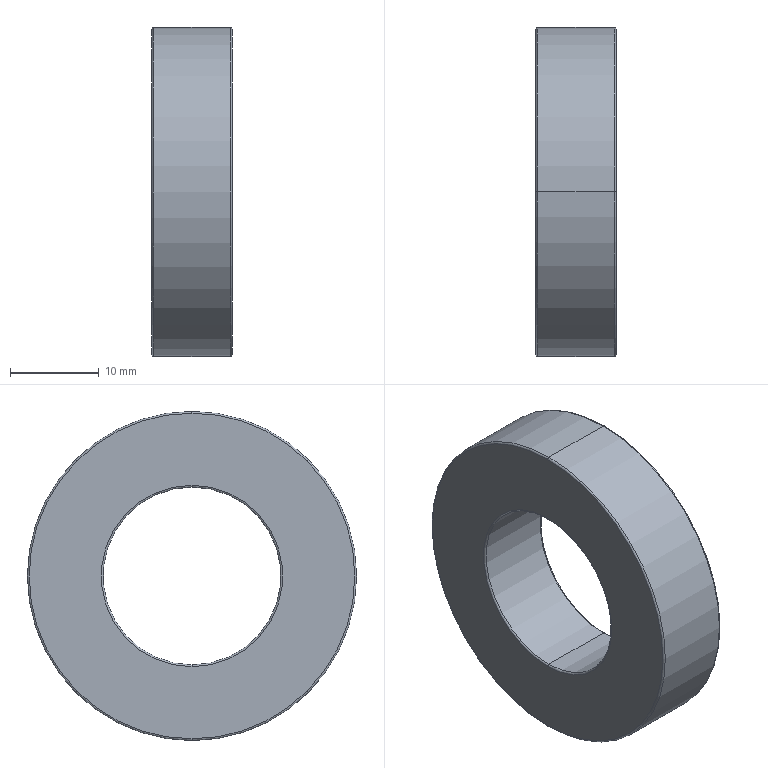Part | SolidWorks | features BaseBody 1 | 1 solid | 14 faces | box 9 x 37 x 37 mm | volume 6846 mm3 | torus 8 | cylinder 4 | plane 2 | commonest cylinder face diameters 20 x2 37 x2
STEP:
#1=CARTESIAN_POINT('',(4.3,0.,18.5));
#2=VERTEX_POINT('',#1);
#3=CARTESIAN_POINT('',(4.3,0.,-18.5));
#4=VERTEX_POINT('',#3);
#5=CARTESIAN_POINT('',(4.3,0.,0.));
#6=DIRECTION('',(-1.,0.,0.));
#7=DIRECTION('',(0.,0.,-1.));
#8=AXIS2_PLACEMENT_3D('',#5,#6,#7);
#9=CIRCLE('',#8,18.5);
#10=EDGE_CURVE('',#2,#4,#9,.T.);
#11=ORIENTED_EDGE('',*,*,#10,.F.);
#12=CARTESIAN_POINT('',(4.5,0.,18.3));
#13=VERTEX_POINT('',#12);
#14=CARTESIAN_POINT('',(4.3,0.,18.3));
#15=DIRECTION('',(0.,1.,0.));
#16=DIRECTION('',(0.,0.,1.));
#17=AXIS2_PLACEMENT_3D('',#14,#15,#16);
#18=CIRCLE('',#17,0.2);
#19=EDGE_CURVE('',#2,#13,#18,.T.);
#20=ORIENTED_EDGE('',*,*,#19,.T.);
#21=CARTESIAN_POINT('',(4.5,0.,-18.3));
#22=VERTEX_POINT('',#21);
#23=CARTESIAN_POINT('',(4.5,0.,0.));
#24=DIRECTION('',(1.,0.,0.));
#25=DIRECTION('',(0.,0.,-1.));
#26=AXIS2_PLACEMENT_3D('',#23,#24,#25);
#27=CIRCLE('',#26,18.3);
#28=EDGE_CURVE('',#22,#13,#27,.T.);
#29=ORIENTED_EDGE('',*,*,#28,.F.);
#30=CARTESIAN_POINT('',(4.3,0.,-18.3));
#31=DIRECTION('',(0.,-1.,0.));
#32=DIRECTION('',(0.,0.,-1.));
#33=AXIS2_PLACEMENT_3D('',#30,#31,#32);
#34=CIRCLE('',#33,0.2);
#35=EDGE_CURVE('',#4,#22,#34,.T.);
#36=ORIENTED_EDGE('',*,*,#35,.F.);
#37=EDGE_LOOP('',(#11,#20,#29,#36));
#38=FACE_OUTER_BOUND('',#37,.T.);
#39=CARTESIAN_POINT('',(4.3,0.,0.));
#40=DIRECTION('',(1.,0.,0.));
#41=DIRECTION('',(0.,0.,-1.));
#42=AXIS2_PLACEMENT_3D('',#39,#40,#41);
#43=TOROIDAL_SURFACE('',#42,18.3,0.2);
#44=ADVANCED_FACE('',(#38),#43,.T.);
#45=CARTESIAN_POINT('',(4.5,0.,10.2));
#46=VERTEX_POINT('',#45);
#47=CARTESIAN_POINT('',(4.5,0.,-10.2));
#48=VERTEX_POINT('',#47);
#49=CARTESIAN_POINT('',(4.5,0.,0.));
#50=DIRECTION('',(-1.,0.,0.));
#51=DIRECTION('',(0.,0.,-1.));
#52=AXIS2_PLACEMENT_3D('',#49,#50,#51);
#53=CIRCLE('',#52,10.2);
#54=EDGE_CURVE('',#46,#48,#53,.T.);
#55=ORIENTED_EDGE('',*,*,#54,.F.);
#56=CARTESIAN_POINT('',(4.3,0.,10.));
#57=VERTEX_POINT('',#56);
#58=CARTESIAN_POINT('',(4.3,0.,10.2));
#59=DIRECTION('',(0.,1.,0.));
#60=DIRECTION('',(0.,0.,1.));
#61=AXIS2_PLACEMENT_3D('',#58,#59,#60);
#62=CIRCLE('',#61,0.2);
#63=EDGE_CURVE('',#46,#57,#62,.T.);
#64=ORIENTED_EDGE('',*,*,#63,.T.);
#65=CARTESIAN_POINT('',(4.3,0.,-10.));
#66=VERTEX_POINT('',#65);
#67=CARTESIAN_POINT('',(4.3,0.,0.));
#68=DIRECTION('',(1.,0.,0.));
#69=DIRECTION('',(0.,0.,-1.));
#70=AXIS2_PLACEMENT_3D('',#67,#68,#69);
#71=CIRCLE('',#70,10.);
#72=EDGE_CURVE('',#66,#57,#71,.T.);
#73=ORIENTED_EDGE('',*,*,#72,.F.);
#74=CARTESIAN_POINT('',(4.3,0.,-10.2));
#75=DIRECTION('',(0.,-1.,0.));
#76=DIRECTION('',(0.,0.,-1.));
#77=AXIS2_PLACEMENT_3D('',#74,#75,#76);
#78=CIRCLE('',#77,0.2);
#79=EDGE_CURVE('',#48,#66,#78,.T.);
#80=ORIENTED_EDGE('',*,*,#79,.F.);
#81=EDGE_LOOP('',(#55,#64,#73,#80));
#82=FACE_OUTER_BOUND('',#81,.T.);
#83=CARTESIAN_POINT('',(4.3,0.,0.));
#84=DIRECTION('',(1.,0.,0.));
#85=DIRECTION('',(0.,0.,-1.));
#86=AXIS2_PLACEMENT_3D('',#83,#84,#85);
#87=TOROIDAL_SURFACE('',#86,10.2,0.2);
#88=ADVANCED_FACE('',(#82),#87,.T.);
#89=CARTESIAN_POINT('',(-4.5,0.,18.3));
#90=VERTEX_POINT('',#89);
#91=CARTESIAN_POINT('',(-4.5,0.,-18.3));
#92=VERTEX_POINT('',#91);
#93=CARTESIAN_POINT('',(-4.5,0.,0.));
#94=DIRECTION('',(-1.,0.,0.));
#95=DIRECTION('',(0.,0.,-1.));
#96=AXIS2_PLACEMENT_3D('',#93,#94,#95);
#97=CIRCLE('',#96,18.3);
#98=EDGE_CURVE('',#90,#92,#97,.T.);
#99=ORIENTED_EDGE('',*,*,#98,.F.);
#100=CARTESIAN_POINT('',(-4.3,0.,18.5));
#101=VERTEX_POINT('',#100);
#102=CARTESIAN_POINT('',(-4.3,0.,18.3));
#103=DIRECTION('',(0.,1.,0.));
#104=DIRECTION('',(0.,0.,1.));
#105=AXIS2_PLACEMENT_3D('',#102,#103,#104);
#106=CIRCLE('',#105,0.2);
#107=EDGE_CURVE('',#90,#101,#106,.T.);
#108=ORIENTED_EDGE('',*,*,#107,.T.);
#109=CARTESIAN_POINT('',(-4.3,0.,-18.5));
#110=VERTEX_POINT('',#109);
#111=CARTESIAN_POINT('',(-4.3,0.,0.));
#112=DIRECTION('',(1.,0.,0.));
#113=DIRECTION('',(0.,0.,-1.));
#114=AXIS2_PLACEMENT_3D('',#111,#112,#113);
#115=CIRCLE('',#114,18.5);
#116=EDGE_CURVE('',#110,#101,#115,.T.);
#117=ORIENTED_EDGE('',*,*,#116,.F.);
#118=CARTESIAN_POINT('',(-4.3,0.,-18.3));
#119=DIRECTION('',(0.,-1.,0.));
#120=DIRECTION('',(0.,0.,-1.));
#121=AXIS2_PLACEMENT_3D('',#118,#119,#120);
#122=CIRCLE('',#121,0.2);
#123=EDGE_CURVE('',#92,#110,#122,.T.);
#124=ORIENTED_EDGE('',*,*,#123,.F.);
#125=EDGE_LOOP('',(#99,#108,#117,#124));
#126=FACE_OUTER_BOUND('',#125,.T.);
#127=CARTESIAN_POINT('',(-4.3,0.,0.));
#128=DIRECTION('',(1.,0.,0.));
#129=DIRECTION('',(0.,0.,-1.));
#130=AXIS2_PLACEMENT_3D('',#127,#128,#129);
#131=TOROIDAL_SURFACE('',#130,18.3,0.2);
#132=ADVANCED_FACE('',(#126),#131,.T.);
#133=CARTESIAN_POINT('',(-4.3,0.,10.));
#134=VERTEX_POINT('',#133);
#135=CARTESIAN_POINT('',(-4.3,0.,-10.));
#136=VERTEX_POINT('',#135);
#137=CARTESIAN_POINT('',(-4.3,0.,0.));
#138=DIRECTION('',(-1.,0.,0.));
#139=DIRECTION('',(0.,0.,-1.));
#140=AXIS2_PLACEMENT_3D('',#137,#138,#139);
#141=CIRCLE('',#140,10.);
#142=EDGE_CURVE('',#134,#136,#141,.T.);
#143=ORIENTED_EDGE('',*,*,#142,.F.);
#144=CARTESIAN_POINT('',(-4.5,0.,10.2));
#145=VERTEX_POINT('',#144);
#146=CARTESIAN_POINT('',(-4.3,0.,10.2));
#147=DIRECTION('',(0.,1.,0.));
#148=DIRECTION('',(0.,0.,1.));
#149=AXIS2_PLACEMENT_3D('',#146,#147,#148);
#150=CIRCLE('',#149,0.2);
#151=EDGE_CURVE('',#134,#145,#150,.T.);
#152=ORIENTED_EDGE('',*,*,#151,.T.);
#153=CARTESIAN_POINT('',(-4.5,0.,-10.2));
#154=VERTEX_POINT('',#153);
#155=CARTESIAN_POINT('',(-4.5,0.,0.));
#156=DIRECTION('',(1.,0.,0.));
#157=DIRECTION('',(0.,0.,-1.));
#158=AXIS2_PLACEMENT_3D('',#155,#156,#157);
#159=CIRCLE('',#158,10.2);
#160=EDGE_CURVE('',#154,#145,#159,.T.);
#161=ORIENTED_EDGE('',*,*,#160,.F.);
#162=CARTESIAN_POINT('',(-4.3,0.,-10.2));
#163=DIRECTION('',(0.,-1.,0.));
#164=DIRECTION('',(0.,0.,-1.));
#165=AXIS2_PLACEMENT_3D('',#162,#163,#164);
#166=CIRCLE('',#165,0.2);
#167=EDGE_CURVE('',#136,#154,#166,.T.);
#168=ORIENTED_EDGE('',*,*,#167,.F.);
#169=EDGE_LOOP('',(#143,#152,#161,#168));
#170=FACE_OUTER_BOUND('',#169,.T.);
#171=CARTESIAN_POINT('',(-4.3,0.,0.));
#172=DIRECTION('',(1.,0.,0.));
#173=DIRECTION('',(0.,0.,-1.));
#174=AXIS2_PLACEMENT_3D('',#171,#172,#173);
#175=TOROIDAL_SURFACE('',#174,10.2,0.2);
#176=ADVANCED_FACE('',(#170),#175,.T.);
#177=CARTESIAN_POINT('',(4.3,0.,0.));
#178=DIRECTION('',(1.,0.,0.));
#179=DIRECTION('',(0.,0.,-1.));
#180=AXIS2_PLACEMENT_3D('',#177,#178,#179);
#181=CIRCLE('',#180,10.);
#182=EDGE_CURVE('',#57,#66,#181,.T.);
#183=ORIENTED_EDGE('',*,*,#182,.T.);
#184=CARTESIAN_POINT('',(4.5,0.,-10.));
#185=DIRECTION('',(-1.,0.,0.));
#186=VECTOR('',#185,1000.);
#187=LINE('',#184,#186);
#188=EDGE_CURVE('',#66,#136,#187,.T.);
#189=ORIENTED_EDGE('',*,*,#188,.T.);
#190=CARTESIAN_POINT('',(-4.3,0.,0.));
#191=DIRECTION('',(-1.,0.,0.));
#192=DIRECTION('',(0.,0.,-1.));
#193=AXIS2_PLACEMENT_3D('',#190,#191,#192);
#194=CIRCLE('',#193,10.);
#195=EDGE_CURVE('',#136,#134,#194,.T.);
#196=ORIENTED_EDGE('',*,*,#195,.T.);
#197=CARTESIAN_POINT('',(4.5,0.,10.));
#198=DIRECTION('',(-1.,0.,0.));
#199=VECTOR('',#198,1000.);
#200=LINE('',#197,#199);
#201=EDGE_CURVE('',#57,#134,#200,.T.);
#202=ORIENTED_EDGE('',*,*,#201,.F.);
#203=EDGE_LOOP('',(#183,#189,#196,#202));
#204=FACE_OUTER_BOUND('',#203,.T.);
#205=CARTESIAN_POINT('',(4.5,0.,0.));
#206=DIRECTION('',(-1.,0.,0.));
#207=DIRECTION('',(0.,0.,1.));
#208=AXIS2_PLACEMENT_3D('',#205,#206,#207);
#209=CYLINDRICAL_SURFACE('',#208,10.);
#210=ADVANCED_FACE('',(#204),#209,.F.);
#211=ORIENTED_EDGE('',*,*,#10,.T.);
#212=CARTESIAN_POINT('',(4.5,0.,-18.5));
#213=DIRECTION('',(-1.,0.,0.));
#214=VECTOR('',#213,1000.);
#215=LINE('',#212,#214);
#216=EDGE_CURVE('',#4,#110,#215,.T.);
#217=ORIENTED_EDGE('',*,*,#216,.T.);
#218=ORIENTED_EDGE('',*,*,#116,.T.);
#219=CARTESIAN_POINT('',(4.5,0.,18.5));
#220=DIRECTION('',(-1.,0.,0.));
#221=VECTOR('',#220,1000.);
#222=LINE('',#219,#221);
#223=EDGE_CURVE('',#2,#101,#222,.T.);
#224=ORIENTED_EDGE('',*,*,#223,.F.);
#225=EDGE_LOOP('',(#211,#217,#218,#224));
#226=FACE_OUTER_BOUND('',#225,.T.);
#227=CARTESIAN_POINT('',(4.5,0.,0.));
#228=DIRECTION('',(-1.,0.,0.));
#229=DIRECTION('',(0.,0.,1.));
#230=AXIS2_PLACEMENT_3D('',#227,#228,#229);
#231=CYLINDRICAL_SURFACE('',#230,18.5);
#232=ADVANCED_FACE('',(#226),#231,.T.);
#233=ORIENTED_EDGE('',*,*,#160,.T.);
#234=CARTESIAN_POINT('',(-4.5,0.,0.));
#235=DIRECTION('',(1.,0.,0.));
#236=DIRECTION('',(0.,0.,-1.));
#237=AXIS2_PLACEMENT_3D('',#234,#235,#236);
#238=CIRCLE('',#237,10.2);
#239=EDGE_CURVE('',#145,#154,#238,.T.);
#240=ORIENTED_EDGE('',*,*,#239,.T.);
#241=EDGE_LOOP('',(#233,#240));
#242=FACE_BOUND('',#241,.T.);
#243=CARTESIAN_POINT('',(-4.5,0.,0.));
#244=DIRECTION('',(-1.,0.,0.));
#245=DIRECTION('',(0.,0.,-1.));
#246=AXIS2_PLACEMENT_3D('',#243,#244,#245);
#247=CIRCLE('',#246,18.3);
#248=EDGE_CURVE('',#92,#90,#247,.T.);
#249=ORIENTED_EDGE('',*,*,#248,.T.);
#250=ORIENTED_EDGE('',*,*,#98,.T.);
#251=EDGE_LOOP('',(#249,#250));
#252=FACE_OUTER_BOUND('',#251,.T.);
#253=CARTESIAN_POINT('',(-4.5,0.,0.));
#254=DIRECTION('',(1.,0.,0.));
#255=DIRECTION('',(0.,1.,0.));
#256=AXIS2_PLACEMENT_3D('',#253,#254,#255);
#257=PLANE('',#256);
#258=ADVANCED_FACE('',(#242,#252),#257,.F.);
#259=CARTESIAN_POINT('',(4.5,0.,0.));
#260=DIRECTION('',(-1.,0.,0.));
#261=DIRECTION('',(0.,0.,-1.));
#262=AXIS2_PLACEMENT_3D('',#259,#260,#261);
#263=CIRCLE('',#262,10.2);
#264=EDGE_CURVE('',#48,#46,#263,.T.);
#265=ORIENTED_EDGE('',*,*,#264,.T.);
#266=ORIENTED_EDGE('',*,*,#54,.T.);
#267=EDGE_LOOP('',(#265,#266));
#268=FACE_BOUND('',#267,.T.);
#269=ORIENTED_EDGE('',*,*,#28,.T.);
#270=CARTESIAN_POINT('',(4.5,0.,0.));
#271=DIRECTION('',(1.,0.,0.));
#272=DIRECTION('',(0.,0.,-1.));
#273=AXIS2_PLACEMENT_3D('',#270,#271,#272);
#274=CIRCLE('',#273,18.3);
#275=EDGE_CURVE('',#13,#22,#274,.T.);
#276=ORIENTED_EDGE('',*,*,#275,.T.);
#277=EDGE_LOOP('',(#269,#276));
#278=FACE_OUTER_BOUND('',#277,.T.);
#279=CARTESIAN_POINT('',(4.5,0.,0.));
#280=DIRECTION('',(1.,0.,0.));
#281=DIRECTION('',(0.,1.,0.));
#282=AXIS2_PLACEMENT_3D('',#279,#280,#281);
#283=PLANE('',#282);
#284=ADVANCED_FACE('',(#268,#278),#283,.T.);
#285=ORIENTED_EDGE('',*,*,#216,.F.);
#286=CARTESIAN_POINT('',(4.3,0.,0.));
#287=DIRECTION('',(-1.,0.,0.));
#288=DIRECTION('',(0.,0.,-1.));
#289=AXIS2_PLACEMENT_3D('',#286,#287,#288);
#290=CIRCLE('',#289,18.5);
#291=EDGE_CURVE('',#4,#2,#290,.T.);
#292=ORIENTED_EDGE('',*,*,#291,.T.);
#293=ORIENTED_EDGE('',*,*,#223,.T.);
#294=CARTESIAN_POINT('',(-4.3,0.,0.));
#295=DIRECTION('',(1.,0.,0.));
#296=DIRECTION('',(0.,0.,-1.));
#297=AXIS2_PLACEMENT_3D('',#294,#295,#296);
#298=CIRCLE('',#297,18.5);
#299=EDGE_CURVE('',#101,#110,#298,.T.);
#300=ORIENTED_EDGE('',*,*,#299,.T.);
#301=EDGE_LOOP('',(#285,#292,#293,#300));
#302=FACE_OUTER_BOUND('',#301,.T.);
#303=CARTESIAN_POINT('',(4.5,0.,0.));
#304=DIRECTION('',(-1.,0.,0.));
#305=DIRECTION('',(0.,0.,1.));
#306=AXIS2_PLACEMENT_3D('',#303,#304,#305);
#307=CYLINDRICAL_SURFACE('',#306,18.5);
#308=ADVANCED_FACE('',(#302),#307,.T.);
#309=ORIENTED_EDGE('',*,*,#188,.F.);
#310=ORIENTED_EDGE('',*,*,#72,.T.);
#311=ORIENTED_EDGE('',*,*,#201,.T.);
#312=ORIENTED_EDGE('',*,*,#142,.T.);
#313=EDGE_LOOP('',(#309,#310,#311,#312));
#314=FACE_OUTER_BOUND('',#313,.T.);
#315=CARTESIAN_POINT('',(4.5,0.,0.));
#316=DIRECTION('',(-1.,0.,0.));
#317=DIRECTION('',(0.,0.,1.));
#318=AXIS2_PLACEMENT_3D('',#315,#316,#317);
#319=CYLINDRICAL_SURFACE('',#318,10.);
#320=ADVANCED_FACE('',(#314),#319,.F.);
#321=ORIENTED_EDGE('',*,*,#151,.F.);
#322=ORIENTED_EDGE('',*,*,#195,.F.);
#323=ORIENTED_EDGE('',*,*,#167,.T.);
#324=ORIENTED_EDGE('',*,*,#239,.F.);
#325=EDGE_LOOP('',(#321,#322,#323,#324));
#326=FACE_OUTER_BOUND('',#325,.T.);
#327=CARTESIAN_POINT('',(-4.3,0.,0.));
#328=DIRECTION('',(1.,0.,0.));
#329=DIRECTION('',(0.,0.,-1.));
#330=AXIS2_PLACEMENT_3D('',#327,#328,#329);
#331=TOROIDAL_SURFACE('',#330,10.2,0.2);
#332=ADVANCED_FACE('',(#326),#331,.T.);
#333=ORIENTED_EDGE('',*,*,#107,.F.);
#334=ORIENTED_EDGE('',*,*,#248,.F.);
#335=ORIENTED_EDGE('',*,*,#123,.T.);
#336=ORIENTED_EDGE('',*,*,#299,.F.);
#337=EDGE_LOOP('',(#333,#334,#335,#336));
#338=FACE_OUTER_BOUND('',#337,.T.);
#339=CARTESIAN_POINT('',(-4.3,0.,0.));
#340=DIRECTION('',(1.,0.,0.));
#341=DIRECTION('',(0.,0.,-1.));
#342=AXIS2_PLACEMENT_3D('',#339,#340,#341);
#343=TOROIDAL_SURFACE('',#342,18.3,0.2);
#344=ADVANCED_FACE('',(#338),#343,.T.);
#345=ORIENTED_EDGE('',*,*,#63,.F.);
#346=ORIENTED_EDGE('',*,*,#264,.F.);
#347=ORIENTED_EDGE('',*,*,#79,.T.);
#348=ORIENTED_EDGE('',*,*,#182,.F.);
#349=EDGE_LOOP('',(#345,#346,#347,#348));
#350=FACE_OUTER_BOUND('',#349,.T.);
#351=CARTESIAN_POINT('',(4.3,0.,0.));
#352=DIRECTION('',(1.,0.,0.));
#353=DIRECTION('',(0.,0.,-1.));
#354=AXIS2_PLACEMENT_3D('',#351,#352,#353);
#355=TOROIDAL_SURFACE('',#354,10.2,0.2);
#356=ADVANCED_FACE('',(#350),#355,.T.);
#357=ORIENTED_EDGE('',*,*,#19,.F.);
#358=ORIENTED_EDGE('',*,*,#291,.F.);
#359=ORIENTED_EDGE('',*,*,#35,.T.);
#360=ORIENTED_EDGE('',*,*,#275,.F.);
#361=EDGE_LOOP('',(#357,#358,#359,#360));
#362=FACE_OUTER_BOUND('',#361,.T.);
#363=CARTESIAN_POINT('',(4.3,0.,0.));
#364=DIRECTION('',(1.,0.,0.));
#365=DIRECTION('',(0.,0.,-1.));
#366=AXIS2_PLACEMENT_3D('',#363,#364,#365);
#367=TOROIDAL_SURFACE('',#366,18.3,0.2);
#368=ADVANCED_FACE('',(#362),#367,.T.);
#369=CLOSED_SHELL('',(#44,#88,#132,#176,#210,#232,#258,#284,#308,#320,#332,#344,#356,#368));
#370=MANIFOLD_SOLID_BREP('',#369);
#371=CARTESIAN_POINT('',(0.,0.,0.));
#372=DIRECTION('',(0.,0.,1.));
#373=DIRECTION('',(1.,0.,0.));
#374=AXIS2_PLACEMENT_3D('',#371,#372,#373);
#375=(LENGTH_UNIT()NAMED_UNIT(*)SI_UNIT(.MILLI.,.METRE.));
#376=UNCERTAINTY_MEASURE_WITH_UNIT(LENGTH_MEASURE(0.00001),#375,'','');
#377=(NAMED_UNIT(*)PLANE_ANGLE_UNIT()SI_UNIT($,.RADIAN.));
#378=(NAMED_UNIT(*)SI_UNIT($,.STERADIAN.)SOLID_ANGLE_UNIT());
#379=(GEOMETRIC_REPRESENTATION_CONTEXT(3)GLOBAL_UNCERTAINTY_ASSIGNED_CONTEXT((#376))GLOBAL_UNIT_ASSIGNED_CONTEXT((#375,#377,#378))REPRESENTATION_CONTEXT('',''));
#380=ADVANCED_BREP_SHAPE_REPRESENTATION('',(#370,#374),#379);